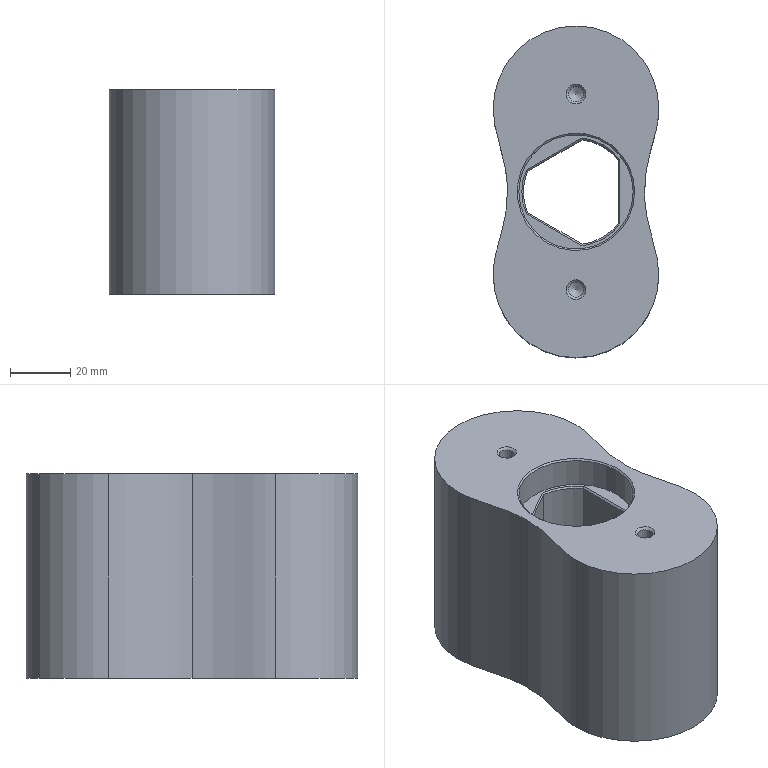NC program | NX | posted with a generic post | part box 55.004 x 110.159 x 68 mm
Lines 1 to 27 of 2889:
N10 G17 G21 G94 G90
(DRILLING_COPY_1 , TOOL : ZXZ)
N12 T01 M6
N14 G54
N16 G17 G0 G90 X-20.25 Y0. S5000 M3
N18 G43 Z30. H1
N20 G94 G81 G98 Z-1. F250. R3.
N22 X20.25
N24 G80
N26 G0 X20.25 Y0. Z30.
N28 M5
(DRILLING_COPY_1_COPY , TOOL : 2.5ZT)
N30 T12 M6
N32 G54
N34 G17 G0 G90 X-20.25 Y0. S2000 M3
N36 G43 Z30. H12
N38 G94 G83 G98 Z-7.751 F120. Q2. R3.
N40 X20.25
N42 G80
N44 G0 X20.25 Y0. Z30.
N46 M5